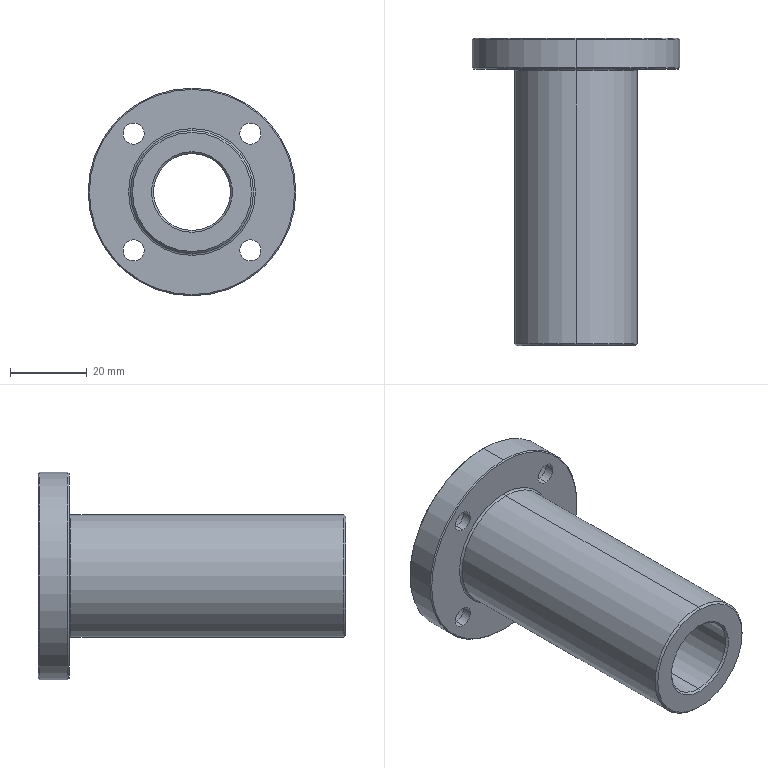Part | STEP file | bearing LMF20LUU | 1 solid | 41 faces | box 54 x 80 x 54 mm | volume 49091 mm3 | cylinder 22 | cone 10 | plane 7 | torus 2 | commonest cylinder face diameters 5.5 x8 10 x8 20 x2 32 x2 54 x2